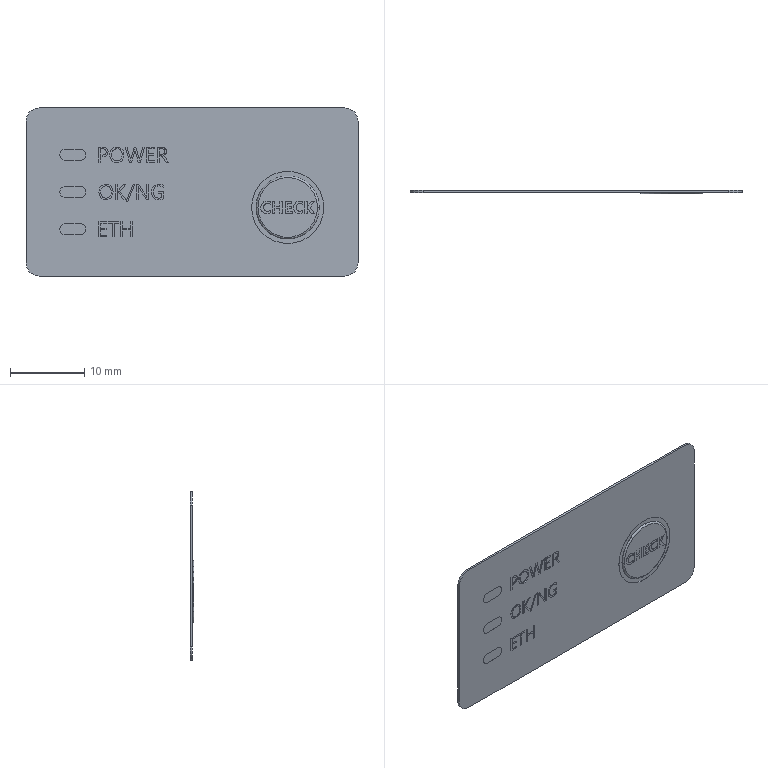Part | SolidWorks | features BaseBody 1 | 1 solid | 315 faces | box 44.6 x 0.5 x 22.6 mm | volume 311.689 mm3 | plane 185 | spline 111 | cylinder 17 | torus 2 | commonest cylinder face diameters 1.5 x9 3.6 x4 8.5 x2 9.7 x2